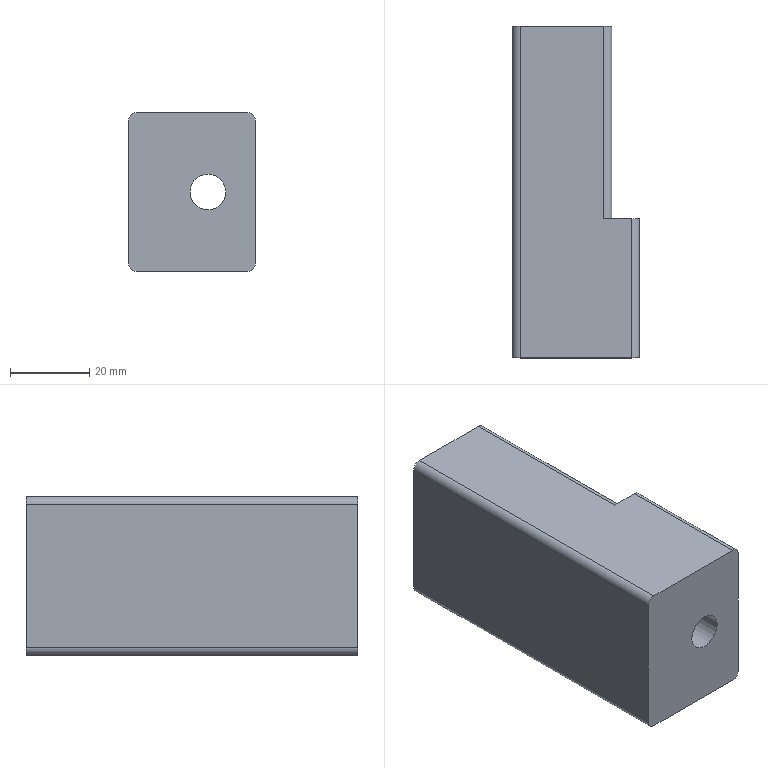NC program | Mastercam | posted with a generic post | part box 32 x 83.5 x 40 mm
Lines 1 to 1602 of 4494:
%
:0001()
(MATERIAL - ALUMINUM MM - 2024)
(T20|63 FEM |H20)
(T9|10 FEM |H9|XY STOCK TO LEAVE - .1|Z STOCK TO LEAVE - 0.)
(T10|10 FEM |H10)
(T18|10 BNOS |H18)
(T15|3 BM/BNOS |H15)
(T5|4 CHM |H5)
(T12|12 FEM |H12|XY STOCK TO LEAVE - .1|Z STOCK TO LEAVE - .1)
(T1|2 FEM |H1)
(T7|6 CHM |H7)
N100 G21
N102 G0 G17 G40 G80 G90 G94 G98
N104 G0 G28 G91 Z0.
N106 G0 G28 X0. Y0.
(63 FEM |TOOL - 20|DIA. OFF. - 20|LEN. - 20|TOOL DIA. - 63.)
N108 T20 M6
N110 G0 G54 G90 X-114.3 Y0. C0. B0. S4000 M3
N112 G43 H20 Z50.
N114 Z2.
N116 G1 Z0. F600.
N118 X114.3 F1000.
N120 G0 Z50.
N122 M5
N124 G0 G28 G91 Z0.
N126 G28
N128 M01
N130 G0 G17 G40 G80 G90 G94 G98
N132 G0 G28 G91 Z0.
(10 FEM |TOOL - 9|DIA. OFF. - 9|LEN. - 9|TOOL DIA. - 10.)
N134 T9 M6
N136 G0 G54 G90 X-42.75 Y27.1 C0. B0. S10000 M3
N138 G43 H9 Z50.
N140 Z1.
N142 G1 Z0. F600.
N144 Y26.1 F5000.
N146 G3 X-41.75 Y25.1 I1.
N148 G1 X41.75 Z-.299
N150 G2 X46.85 Y20. Z-.328 J-5.1
N152 G1 Y-20. Z-.471
N154 G2 X41.75 Y-25.1 Z-.5 I-5.1
N156 G1 X-41.75 Z-.799
N158 G2 X-46.85 Y-20. Z-.828 J5.1
N160 G1 Y20. Z-.971
N162 G2 X-41.75 Y25.1 Z-1. I5.1
N164 G1 X41.75 Z-1.299
N166 G2 X46.85 Y20. Z-1.328 J-5.1
N168 G1 Y-20. Z-1.471
N170 G2 X41.75 Y-25.1 Z-1.5 I-5.1
N172 G1 X-41.75 Z-1.799
N174 G2 X-46.85 Y-20. Z-1.828 J5.1
N176 G1 Y20. Z-1.971
N178 G2 X-41.75 Y25.1 Z-2. I5.1
N180 G1 X41.75 Z-2.299
N182 G2 X46.85 Y20. Z-2.328 J-5.1
N184 G1 Y-20. Z-2.471
N186 G2 X41.75 Y-25.1 Z-2.5 I-5.1
N188 G1 X-41.75 Z-2.799
N190 G2 X-46.85 Y-20. Z-2.828 J5.1
N192 G1 Y20. Z-2.971
N194 G2 X-41.75 Y25.1 Z-3. I5.1
N196 G1 X41.75 Z-3.299
N198 G2 X46.85 Y20. Z-3.328 J-5.1
N200 G1 Y-20. Z-3.471
N202 G2 X41.75 Y-25.1 Z-3.5 I-5.1
N204 G1 X-41.75 Z-3.799
N206 G2 X-46.85 Y-20. Z-3.828 J5.1
N208 G1 Y20. Z-3.971
N210 G2 X-41.75 Y25.1 Z-4. I5.1
N212 G1 X41.75 Z-4.299
N214 G2 X46.85 Y20. Z-4.328 J-5.1
N216 G1 Y-20. Z-4.471
N218 G2 X41.75 Y-25.1 Z-4.5 I-5.1
N220 G1 X-41.75 Z-4.799
N222 G2 X-46.85 Y-20. Z-4.828 J5.1
N224 G1 Y20. Z-4.971
N226 G2 X-41.75 Y25.1 Z-5. I5.1
N228 G1 X41.75 Z-5.299
N230 G2 X46.85 Y20. Z-5.328 J-5.1
N232 G1 Y-20. Z-5.471
N234 G2 X41.75 Y-25.1 Z-5.5 I-5.1
N236 G1 X-41.75 Z-5.799
N238 G2 X-46.85 Y-20. Z-5.828 J5.1
N240 G1 Y20. Z-5.971
N242 G2 X-41.75 Y25.1 Z-6. I5.1
N244 G1 X41.75 Z-6.299
N246 G2 X46.85 Y20. Z-6.328 J-5.1
N248 G1 Y-20. Z-6.471
N250 G2 X41.75 Y-25.1 Z-6.5 I-5.1
N252 G1 X-41.75 Z-6.799
N254 G2 X-46.85 Y-20. Z-6.828 J5.1
N256 G1 Y20. Z-6.971
N258 G2 X-41.75 Y25.1 Z-7. I5.1
N260 G1 X41.75 Z-7.299
N262 G2 X46.85 Y20. Z-7.328 J-5.1
N264 G1 Y-20. Z-7.471
N266 G2 X41.75 Y-25.1 Z-7.5 I-5.1
N268 G1 X-41.75 Z-7.799
N270 G2 X-46.85 Y-20. Z-7.828 J5.1
N272 G1 Y20. Z-7.971
N274 G2 X-41.75 Y25.1 Z-8. I5.1
N276 G1 X41.75 Z-8.299
N278 G2 X46.85 Y20. Z-8.328 J-5.1
N280 G1 Y-20. Z-8.471
N282 G2 X41.75 Y-25.1 Z-8.5 I-5.1
N284 G1 X-41.75 Z-8.799
N286 G2 X-46.85 Y-20. Z-8.828 J5.1
N288 G1 Y20. Z-8.971
N290 G2 X-41.75 Y25.1 Z-9. I5.1
N292 G1 X41.75 Z-9.299
N294 G2 X46.85 Y20. Z-9.328 J-5.1
N296 G1 Y-20. Z-9.471
N298 G2 X41.75 Y-25.1 Z-9.5 I-5.1
N300 G1 X-41.75 Z-9.799
N302 G2 X-46.85 Y-20. Z-9.828 J5.1
N304 G1 Y20. Z-9.971
N306 G2 X-41.75 Y25.1 Z-10. I5.1
N308 G1 X41.75 Z-10.299
N310 G2 X46.85 Y20. Z-10.328 J-5.1
N312 G1 Y-20. Z-10.471
N314 G2 X41.75 Y-25.1 Z-10.5 I-5.1
N316 G1 X-41.75 Z-10.799
N318 G2 X-46.85 Y-20. Z-10.828 J5.1
N320 G1 Y20. Z-10.971
N322 G2 X-41.75 Y25.1 Z-11. I5.1
N324 G1 X41.75 Z-11.299
N326 G2 X46.85 Y20. Z-11.328 J-5.1
N328 G1 Y-20. Z-11.471
N330 G2 X41.75 Y-25.1 Z-11.5 I-5.1
N332 G1 X-41.75 Z-11.799
N334 G2 X-46.85 Y-20. Z-11.828 J5.1
N336 G1 Y20. Z-11.971
N338 G2 X-41.75 Y25.1 Z-12. I5.1
N340 G1 X41.75 Z-12.299
N342 G2 X46.85 Y20. Z-12.328 J-5.1
N344 G1 Y-20. Z-12.471
N346 G2 X41.75 Y-25.1 Z-12.5 I-5.1
N348 G1 X-41.75 Z-12.799
N350 G2 X-46.85 Y-20. Z-12.828 J5.1
N352 G1 Y20. Z-12.971
N354 G2 X-41.75 Y25.1 Z-13. I5.1
N356 G1 X41.75 Z-13.299
N358 G2 X46.85 Y20. Z-13.328 J-5.1
N360 G1 Y-20. Z-13.471
N362 G2 X41.75 Y-25.1 Z-13.5 I-5.1
N364 G1 X-41.75 Z-13.799
N366 G2 X-46.85 Y-20. Z-13.828 J5.1
N368 G1 Y20. Z-13.971
N370 G2 X-41.75 Y25.1 Z-14. I5.1
N372 G1 X41.75 Z-14.299
N374 G2 X46.85 Y20. Z-14.328 J-5.1
N376 G1 Y-20. Z-14.471
N378 G2 X41.75 Y-25.1 Z-14.5 I-5.1
N380 G1 X-41.75 Z-14.799
N382 G2 X-46.85 Y-20. Z-14.828 J5.1
N384 G1 Y20. Z-14.971
N386 G2 X-41.75 Y25.1 Z-15. I5.1
N388 G1 X41.75 Z-15.299
N390 G2 X46.85 Y20. Z-15.328 J-5.1
N392 G1 Y-20. Z-15.471
N394 G2 X41.75 Y-25.1 Z-15.5 I-5.1
N396 G1 X-41.75 Z-15.799
N398 G2 X-46.85 Y-20. Z-15.828 J5.1
N400 G1 Y20. Z-15.971
N402 G2 X-41.75 Y25.1 Z-16. I5.1
N404 G1 X41.75 Z-16.299
N406 G2 X46.85 Y20. Z-16.328 J-5.1
N408 G1 Y-20. Z-16.471
N410 G2 X41.75 Y-25.1 Z-16.5 I-5.1
N412 G1 X-41.75 Z-16.799
N414 G2 X-46.85 Y-20. Z-16.828 J5.1
N416 G1 Y20. Z-16.971
N418 G2 X-41.75 Y25.1 Z-17. I5.1
N420 G1 X41.75 Z-17.299
N422 G2 X46.85 Y20. Z-17.328 J-5.1
N424 G1 Y-20. Z-17.471
N426 G2 X41.75 Y-25.1 Z-17.5 I-5.1
N428 G1 X-41.75 Z-17.799
N430 G2 X-46.85 Y-20. Z-17.828 J5.1
N432 G1 Y20. Z-17.971
N434 G2 X-41.75 Y25.1 Z-18. I5.1
N436 G1 X41.75 Z-18.299
N438 G2 X46.85 Y20. Z-18.328 J-5.1
N440 G1 Y-20. Z-18.471
N442 G2 X41.75 Y-25.1 Z-18.5 I-5.1
N444 G1 X-41.75 Z-18.799
N446 G2 X-46.85 Y-20. Z-18.828 J5.1
N448 G1 Y20. Z-18.971
N450 G2 X-41.75 Y25.1 Z-19. I5.1
N452 G1 X41.75 Z-19.299
N454 G2 X46.85 Y20. Z-19.328 J-5.1
N456 G1 Y-20. Z-19.471
N458 G2 X41.75 Y-25.1 Z-19.5 I-5.1
N460 G1 X-41.75 Z-19.799
N462 G2 X-46.85 Y-20. Z-19.828 J5.1
N464 G1 Y20. Z-19.971
N466 G2 X-41.75 Y25.1 Z-20. I5.1
N468 G1 X41.75 Z-20.299
N470 G2 X46.85 Y20. Z-20.328 J-5.1
N472 G1 Y-20. Z-20.471
N474 G2 X41.75 Y-25.1 Z-20.5 I-5.1
N476 G1 X-41.75 Z-20.799
N478 G2 X-46.85 Y-20. Z-20.828 J5.1
N480 G1 Y20. Z-20.971
N482 G2 X-41.75 Y25.1 Z-21. I5.1
N484 G1 X41.75 Z-21.299
N486 G2 X46.85 Y20. Z-21.328 J-5.1
N488 G1 Y-20. Z-21.471
N490 G2 X41.75 Y-25.1 Z-21.5 I-5.1
N492 G1 X-41.75 Z-21.799
N494 G2 X-46.85 Y-20. Z-21.828 J5.1
N496 G1 Y20. Z-21.971
N498 G2 X-41.75 Y25.1 Z-22. I5.1
N500 G1 X41.75 Z-22.299
N502 G2 X46.85 Y20. Z-22.328 J-5.1
N504 G1 Y-20. Z-22.471
N506 G2 X41.75 Y-25.1 Z-22.5 I-5.1
N508 G1 X-41.75 Z-22.799
N510 G2 X-46.85 Y-20. Z-22.828 J5.1
N512 G1 Y20. Z-22.971
N514 G2 X-41.75 Y25.1 Z-23. I5.1
N516 G1 X41.75 Z-23.299
N518 G2 X46.85 Y20. Z-23.328 J-5.1
N520 G1 Y-20. Z-23.471
N522 G2 X41.75 Y-25.1 Z-23.5 I-5.1
N524 G1 X-41.75 Z-23.799
N526 G2 X-46.85 Y-20. Z-23.828 J5.1
N528 G1 Y20. Z-23.971
N530 G2 X-41.75 Y25.1 Z-24. I5.1
N532 G1 X41.75 Z-24.299
N534 G2 X46.85 Y20. Z-24.328 J-5.1
N536 G1 Y-20. Z-24.471
N538 G2 X41.75 Y-25.1 Z-24.5 I-5.1
N540 G1 X-41.75 Z-24.799
N542 G2 X-46.85 Y-20. Z-24.828 J5.1
N544 G1 Y20. Z-24.971
N546 G2 X-41.75 Y25.1 Z-25. I5.1
N548 G1 X41.75 Z-25.299
N550 G2 X46.85 Y20. Z-25.328 J-5.1
N552 G1 Y-20. Z-25.471
N554 G2 X41.75 Y-25.1 Z-25.5 I-5.1
N556 G1 X-41.75 Z-25.799
N558 G2 X-46.85 Y-20. Z-25.828 J5.1
N560 G1 Y20. Z-25.971
N562 G2 X-41.75 Y25.1 Z-26. I5.1
N564 G1 X41.75 Z-26.299
N566 G2 X46.85 Y20. Z-26.328 J-5.1
N568 G1 Y-20. Z-26.471
N570 G2 X41.75 Y-25.1 Z-26.5 I-5.1
N572 G1 X-41.75 Z-26.799
N574 G2 X-46.85 Y-20. Z-26.828 J5.1
N576 G1 Y20. Z-26.971
N578 G2 X-41.75 Y25.1 Z-27. I5.1
N580 G1 X41.75 Z-27.299
N582 G2 X46.85 Y20. Z-27.328 J-5.1
N584 G1 Y-20. Z-27.471
N586 G2 X41.75 Y-25.1 Z-27.5 I-5.1
N588 G1 X-41.75 Z-27.799
N590 G2 X-46.85 Y-20. Z-27.828 J5.1
N592 G1 Y20. Z-27.971
N594 G2 X-41.75 Y25.1 Z-28. I5.1
N596 G1 X41.75 Z-28.299
N598 G2 X46.85 Y20. Z-28.328 J-5.1
N600 G1 Y-20. Z-28.471
N602 G2 X41.75 Y-25.1 Z-28.5 I-5.1
N604 G1 X-41.75 Z-28.799
N606 G2 X-46.85 Y-20. Z-28.828 J5.1
N608 G1 Y20. Z-28.971
N610 G2 X-41.75 Y25.1 Z-29. I5.1
N612 G1 X41.75 Z-29.299
N614 G2 X46.85 Y20. Z-29.328 J-5.1
N616 G1 Y-20. Z-29.471
N618 G2 X41.75 Y-25.1 Z-29.5 I-5.1
N620 G1 X-41.75 Z-29.799
N622 G2 X-46.85 Y-20. Z-29.828 J5.1
N624 G1 Y20. Z-29.971
N626 G2 X-41.75 Y25.1 Z-30. I5.1
N628 G1 X41.75 Z-30.299
N630 G2 X46.85 Y20. Z-30.328 J-5.1
N632 G1 Y-20. Z-30.471
N634 G2 X41.75 Y-25.1 Z-30.5 I-5.1
N636 G1 X-41.75 Z-30.799
N638 G2 X-46.85 Y-20. Z-30.828 J5.1
N640 G1 Y20. Z-30.971
N642 G2 X-41.75 Y25.1 Z-31. I5.1
N644 G1 X41.75 Z-31.299
N646 G2 X46.85 Y20. Z-31.328 J-5.1
N648 G1 Y-20. Z-31.471
N650 G2 X41.75 Y-25.1 Z-31.5 I-5.1
N652 G1 X-41.75 Z-31.799
N654 G2 X-46.85 Y-20. Z-31.828 J5.1
N656 G1 Y20. Z-31.971
N658 G2 X-41.75 Y25.1 Z-32. I5.1
N660 G1 X41.75 Z-32.299
N662 G2 X46.85 Y20. Z-32.328 J-5.1
N664 G1 Y-20. Z-32.471
N666 G2 X41.75 Y-25.1 Z-32.5 I-5.1
N668 G1 X-41.75
N670 G2 X-46.85 Y-20. J5.1
N672 G1 Y20.
N674 G2 X-41.75 Y25.1 I5.1
N676 G1 X41.75
N678 G2 X46.85 Y20. J-5.1
N680 G1 Y-20.
N682 G2 X41.75 Y-25.1 I-5.1
N684 G3 X40.75 Y-26.1 J-1.
N686 G1 Y-27.1
N688 G0 Z50.
N690 M5
N692 G0 G28 G91 Z0.
N694 G28
N696 M01
N698 G0 G17 G40 G80 G90 G94 G98
N700 G0 G28 G91 Z0.
(10 FEM |TOOL - 10|DIA. OFF. - 10|LEN. - 10|TOOL DIA. - 10.)
N702 T10 M6
N704 G0 G54 G90 X-46.75 Y-25.002 C0. B0. S7000 M3
N706 G43 H10 Z50.
N708 Z1.
N710 G1 Z-16.25 F600.
N712 Y-.002 F1000.
N714 Y20.
N716 G2 X-41.75 Y25. I5.
N718 G1 X41.75
N720 G2 X46.75 Y20. J-5.
N722 G1 Y-20.
N724 G2 X41.75 Y-25. I-5.
N726 G1 X-41.75
N728 G2 X-46.75 Y-20. J5.
N730 G1 Y-.002
N732 Y24.998
N734 G0 Z50.
N736 Y-25.002
N738 Z-15.25
N740 G1 Z-32.5 F600.
N742 Y-.002 F1000.
N744 Y20.
N746 G2 X-41.75 Y25. I5.
N748 G1 X41.75
N750 G2 X46.75 Y20. J-5.
N752 G1 Y-20.
N754 G2 X41.75 Y-25. I-5.
N756 G1 X-41.75
N758 G2 X-46.75 Y-20. J5.
N760 G1 Y-.002
N762 Y24.998
N764 G0 Z50.
N766 M5
N768 G0 G28 G91 Z0.
N770 G28
N772 M01
N774 G0 G17 G40 G80 G90 G94 G98
N776 G0 G28 G91 Z0.
(10 BNOS |TOOL - 18|DIA. OFF. - 18|LEN. - 18|TOOL DIA. - 10.)
N778 T18 M6
N780 G0 G54 G90 X46.75 Y22. C0. B0. S7000 M3
N782 G43 H18 Z50.
N784 Z5.
N786 G1 Z0. F600.
N788 X41.75 F3000.
N790 X-41.75
N792 X-46.75
N794 Y22.134
N796 Z-.003
N798 X-41.75
N800 X41.75
N802 X46.75
N804 Y22.27
N806 Z-.012
N808 X41.75
N810 X-41.75
N812 X-46.75
N814 Y22.407
N816 Z-.028
N818 X-41.75
N820 X41.75
N822 X46.75
N824 Y22.546
N826 Z-.05
N828 X41.75
N830 X-41.75
N832 X-46.75
N834 Y22.686
N836 Z-.079
N838 X-41.75
N840 X41.75
N842 X46.75
N844 Y22.825
N846 Z-.116
N848 X41.75
N850 X-41.75
N852 X-46.75
N854 Y22.965
N856 Z-.16
N858 X-41.75
N860 X41.75
N862 X46.75
N864 Y23.104
N866 Z-.211
N868 X41.75
N870 X-41.75
N872 X-46.75
N874 Y23.227
N876 Z-.262
N878 X-41.75
N880 X41.75
N882 X46.75
N884 Y23.348
N886 Z-.32
N888 X41.75
N890 X-41.75
N892 X-46.75
N894 Y23.467
N896 Z-.383
N898 X-41.75
N900 X41.75
N902 X46.75
N904 Y23.584
N906 Z-.452
N908 X41.75
N910 X-41.75
N912 X-46.75
N914 Y23.698
N916 Z-.527
N918 X-41.75
N920 X41.75
N922 X46.75
N924 Y23.81
N926 Z-.607
N928 X41.75
N930 X-41.75
N932 X-46.75
N934 Y23.918
N936 Z-.693
N938 X-41.75
N940 X41.75
N942 X46.75
N944 Y24.021
N946 Z-.783
N948 X41.75
N950 X-41.75
N952 X-46.75
N954 Y24.121
N956 Z-.879
N958 X-41.75
N960 X41.75
N962 X46.75
N964 Y24.217
N966 Z-.979
N968 X41.75
N970 X-41.75
N972 X-46.75
N974 Y24.307
N976 Z-1.082
N978 X-41.75
N980 X41.75
N982 X46.75
N984 Y24.393
N986 Z-1.19
N988 X41.75
N990 X-41.75
N992 X-46.75
N994 Y24.473
N996 Z-1.302
N998 X-41.75
N1000 X41.75
N1002 X46.75
N1004 Y24.548
N1006 Z-1.416
N1008 X41.75
N1010 X-41.75
N1012 X-46.75
N1014 Y24.617
N1016 Z-1.533
N1018 X-41.75
N1020 X41.75
N1022 X46.75
N1024 Y24.68
N1026 Z-1.652
N1028 X41.75
N1030 X-41.75
N1032 X-46.75
N1034 Y24.738
N1036 Z-1.773
N1038 X-41.75
N1040 X41.75
N1042 X46.75
N1044 Y24.789
N1046 Z-1.896
N1048 X41.75
N1050 X-41.75
N1052 X-46.75
N1054 Y24.84
N1056 Z-2.035
N1058 X-41.75
N1060 X41.75
N1062 X46.75
N1064 Y24.884
N1066 Z-2.175
N1068 X41.75
N1070 X-41.75
N1072 X-46.75
N1074 Y24.921
N1076 Z-2.314
N1078 X-41.75
N1080 X41.75
N1082 X46.75
N1084 Y24.95
N1086 Z-2.454
N1088 X41.75
N1090 X-41.75
N1092 X-46.75
N1094 Y24.972
N1096 Z-2.593
N1098 X-41.75
N1100 X41.75
N1102 X46.75
N1104 Y24.988
N1106 Z-2.73
N1108 X41.75
N1110 X-41.75
N1112 X-46.75
N1114 Y24.997
N1116 Z-2.866
N1118 X-41.75
N1120 X41.75
N1122 X46.75
N1124 Y25.
N1126 Z-3.
N1128 X41.75
N1130 X-41.75
N1132 X-46.75
N1134 G0 Z2.
N1136 Z50.
N1138 Y-25.
N1140 Z2.
N1142 G1 Z-3. F600.
N1144 X-41.75 F3000.
N1146 X41.75
N1148 X46.75
N1150 Z-2.866
N1152 Y-24.997
N1154 X41.75
N1156 X-41.75
N1158 X-46.75
N1160 Z-2.73
N1162 Y-24.988
N1164 X-41.75
N1166 X41.75
N1168 X46.75
N1170 Z-2.593
N1172 Y-24.972
N1174 X41.75
N1176 X-41.75
N1178 X-46.75
N1180 Z-2.454
N1182 Y-24.95
N1184 X-41.75
N1186 X41.75
N1188 X46.75
N1190 Z-2.314
N1192 Y-24.921
N1194 X41.75
N1196 X-41.75
N1198 X-46.75
N1200 Z-2.175
N1202 Y-24.884
N1204 X-41.75
N1206 X41.75
N1208 X46.75
N1210 Z-2.035
N1212 Y-24.84
N1214 X41.75
N1216 X-41.75
N1218 X-46.75
N1220 Z-1.896
N1222 Y-24.789
N1224 X-41.75
N1226 X41.75
N1228 X46.75
N1230 Z-1.773
N1232 Y-24.738
N1234 X41.75
N1236 X-41.75
N1238 X-46.75
N1240 Z-1.652
N1242 Y-24.68
N1244 X-41.75
N1246 X41.75
N1248 X46.75
N1250 Z-1.533
N1252 Y-24.617
N1254 X41.75
N1256 X-41.75
N1258 X-46.75
N1260 Z-1.416
N1262 Y-24.548
N1264 X-41.75
N1266 X41.75
N1268 X46.75
N1270 Z-1.302
N1272 Y-24.473
N1274 X41.75
N1276 X-41.75
N1278 X-46.75
N1280 Z-1.19
N1282 Y-24.393
N1284 X-41.75
N1286 X41.75
N1288 X46.75
N1290 Z-1.082
N1292 Y-24.307
N1294 X41.75
N1296 X-41.75
N1298 X-46.75
N1300 Z-.979
N1302 Y-24.217
N1304 X-41.75
N1306 X41.75
N1308 X46.75
N1310 Z-.879
N1312 Y-24.121
N1314 X41.75
N1316 X-41.75
N1318 X-46.75
N1320 Z-.783
N1322 Y-24.021
N1324 X-41.75
N1326 X41.75
N1328 X46.75
N1330 Z-.693
N1332 Y-23.918
N1334 X41.75
N1336 X-41.75
N1338 X-46.75
N1340 Z-.607
N1342 Y-23.81
N1344 X-41.75
N1346 X41.75
N1348 X46.75
N1350 Z-.527
N1352 Y-23.698
N1354 X41.75
N1356 X-41.75
N1358 X-46.75
N1360 Z-.452
N1362 Y-23.584
N1364 X-41.75
N1366 X41.75
N1368 X46.75
N1370 Z-.383
N1372 Y-23.467
N1374 X41.75
N1376 X-41.75
N1378 X-46.75
N1380 Z-.32
N1382 Y-23.348
N1384 X-41.75
N1386 X41.75
N1388 X46.75
N1390 Z-.262
N1392 Y-23.227
N1394 X41.75
N1396 X-41.75
N1398 X-46.75
N1400 Z-.211
N1402 Y-23.104
N1404 X-41.75
N1406 X41.75
N1408 X46.75
N1410 Z-.16
N1412 Y-22.965
N1414 X41.75
N1416 X-41.75
N1418 X-46.75
N1420 Z-.116
N1422 Y-22.825
N1424 X-41.75
N1426 X41.75
N1428 X46.75
N1430 Z-.079
N1432 Y-22.686
N1434 X41.75
N1436 X-41.75
N1438 X-46.75
N1440 Z-.05
N1442 Y-22.546
N1444 X-41.75
N1446 X41.75
N1448 X46.75
N1450 Z-.028
N1452 Y-22.407
N1454 X41.75
N1456 X-41.75
N1458 X-46.75
N1460 Z-.012
N1462 Y-22.27
N1464 X-41.75
N1466 X41.75
N1468 X46.75
N1470 Z-.003
N1472 Y-22.134
N1474 X41.75
N1476 X-41.75
N1478 X-46.75
N1480 Z0.
N1482 Y-22.
N1484 X-41.75
N1486 X41.75
N1488 X46.75
N1490 G0 Z5.
N1492 Z50.
N1494 M5
N1496 G0 G28 G91 Z0.
N1498 G28
N1500 M01
N1502 G0 G17 G40 G80 G90 G94 G98
N1504 G0 G28 G91 Z0.
(3 BM/BNOS |TOOL - 15|DIA. OFF. - 15|LEN. - 15|TOOL DIA. - 3.)
N1506 T15 M6
N1508 G0 G54 G90 X43.906 Y22.212 C0. B0. S7000 M3
N1510 G43 H15 Z50.
N1512 Z16.225
N1514 Z6.225
N1516 G1 Z-3.775 F600.
N1518 X43.887 Y22.194 Z-3.92 F1000.
N1520 X43.836 Y22.142 Z-4.051
N1522 X43.758 Y22.064 Z-4.167
N1524 X43.66 Y21.966 Z-4.266
N1526 X43.548 Y21.855 Z-4.347
N1528 X43.43 Y21.737 Z-4.407
N1530 X43.311 Y21.618 Z-4.445
N1532 X43.199 Y21.506 Z-4.46
N1534 X43.096 Y21.401 Z-4.437
N1536 X43.003 Y21.304 Z-4.366
N1538 X42.922 Y21.217 Z-4.259
N1540 X42.853 Y21.14 Z-4.122
N1542 X42.797 Y21.075 Z-3.967
N1544 X42.756 Y21.024 Z-3.801
N1546 X42.73 Y20.988 Z-3.634
N1548 X42.72 Y20.969 Z-3.475
N1550 X42.719 Y20.959 Z-3.327
N1552 X42.72 Y20.956 Z-3.253
N1554 X42.719 Y20.951 Z-3.179
N1556 Y20.927 Z-3.029
N1558 X42.72 Y20.915 Z-2.954
N1560 X42.719 Y20.902 Z-2.88
N1562 X42.721 Y20.864 Z-2.731
N1564 X42.72 Y20.823 Z-2.582
N1566 X42.721 Y20.768 Z-2.438
N1568 Y20.712 Z-2.294
N1570 Y20.642 Z-2.156
N1572 Y20.572 Z-2.018
N1574 Y20.488 Z-1.888
N1576 Y20.402 Z-1.757
N1578 Y20.305 Z-1.636
N1580 X42.72 Y20.206 Z-1.515
N1582 X42.721 Y20.096 Z-1.404
N1584 X42.72 Y19.985 Z-1.294
N1586 X42.721 Y19.864 Z-1.195
N1588 Y19.743 Z-1.098
N1590 Y19.613 Z-1.012
N1592 Y19.482 Z-.928
N1594 Y19.344 Z-.858
N1596 Y19.206 Z-.788
N1598 Y19.062 Z-.732
N1600 X42.72 Y18.918 Z-.677
N1602 X42.721 Y18.769 Z-.636
N1604 X42.719 Y18.62 Z-.598
N1606 X42.72 Y18.546 Z-.585
N1608 X42.719 Y18.471 Z-.573
N1610 Y18.321 Z-.549
N1612 X42.72 Y18.247 Z-.544
N1614 X42.719 Y18.173 Z-.541
N1616 Y18.025 Z-.531
N1618 Y16.8
N1620 Y15.6
N1622 Y14.4
N1624 Y13.2
N1626 Y12.
N1628 Y10.8
N1630 Y9.6
N1632 Y8.4
N1634 Y7.2
N1636 Y6.
N1638 Y4.8
N1640 Y3.6
N1642 Y2.4
N1644 Y1.2
N1646 Y0.
N1648 Y-1.2
N1650 Y-2.4
N1652 Y-3.6
N1654 Y-4.8
N1656 Y-6.
N1658 Y-7.2
N1660 Y-8.4
N1662 Y-9.6
N1664 Y-10.8
N1666 Y-12.
N1668 Y-13.2
N1670 Y-14.4
N1672 Y-15.6
N1674 Y-16.8
N1676 X42.72 Y-18.025
N1678 X42.719 Y-18.173 Z-.541
N1680 X42.72 Y-18.247 Z-.544
N1682 X42.719 Y-18.321 Z-.549
N1684 Y-18.471 Z-.573
N1686 X42.72 Y-18.546 Z-.585
N1688 X42.719 Y-18.62 Z-.598
N1690 X42.721 Y-18.769 Z-.636
N1692 X42.72 Y-18.918 Z-.677
N1694 X42.721 Y-19.062 Z-.732
N1696 Y-19.206 Z-.788
N1698 Y-19.344 Z-.858
N1700 Y-19.482 Z-.928
N1702 Y-19.612 Z-1.012
N1704 Y-19.743 Z-1.098
N1706 Y-19.864 Z-1.195
N1708 X42.72 Y-19.985 Z-1.294
N1710 X42.721 Y-20.096 Z-1.404
N1712 X42.72 Y-20.206 Z-1.515
N1714 X42.721 Y-20.305 Z-1.636
N1716 Y-20.402 Z-1.757
N1718 Y-20.488 Z-1.888
N1720 Y-20.572 Z-2.018
N1722 Y-20.642 Z-2.156
N1724 Y-20.712 Z-2.294
N1726 Y-20.768 Z-2.438
N1728 X42.72 Y-20.823 Z-2.582
N1730 X42.721 Y-20.864 Z-2.731
N1732 X42.719 Y-20.902 Z-2.88
N1734 X42.72 Y-20.915 Z-2.954
N1736 X42.719 Y-20.927 Z-3.029
N1738 Y-20.951 Z-3.179
N1740 X42.72 Y-20.956 Z-3.253
N1742 X42.719 Y-20.959 Z-3.327
N1744 Y-20.968 Z-3.475
N1746 X42.728 Y-20.986 Z-3.633
N1748 X42.753 Y-21.021 Z-3.8
N1750 X42.793 Y-21.071 Z-3.966
N1752 X42.848 Y-21.135 Z-4.122
N1754 X42.917 Y-21.212 Z-4.259
N1756 X42.997 Y-21.299 Z-4.367
N1758 X43.089 Y-21.395 Z-4.437
N1760 X43.192 Y-21.499 Z-4.461
N1762 X43.304 Y-21.611 Z-4.446
N1764 X43.423 Y-21.73 Z-4.407
N1766 X43.541 Y-21.848 Z-4.347
N1768 X43.653 Y-21.959 Z-4.267
N1770 X43.751 Y-22.057 Z-4.168
N1772 X43.829 Y-22.135 Z-4.052
N1774 X43.881 Y-22.187 Z-3.92
N1776 X43.899 Y-22.206 Z-3.775
N1778 G0 Z6.225
N1780 Z16.225
N1782 Z50.
N1784 X-43.896 Y-22.202
N1786 Z16.224
N1788 Z6.224
N1790 G1 Z-3.776 F600.
N1792 X-43.877 Y-22.183 Z-3.921 F1000.
N1794 X-43.825 Y-22.132 Z-4.052
N1796 X-43.747 Y-22.054 Z-4.168
N1798 X-43.649 Y-21.956 Z-4.267
N1800 X-43.538 Y-21.844 Z-4.347
N1802 X-43.419 Y-21.726 Z-4.407
N1804 X-43.301 Y-21.608 Z-4.446
N1806 X-43.188 Y-21.495 Z-4.461
N1808 X-43.086 Y-21.392 Z-4.437
N1810 X-42.994 Y-21.296 Z-4.367
N1812 X-42.914 Y-21.209 Z-4.258
N1814 X-42.846 Y-21.133 Z-4.122
N1816 X-42.792 Y-21.07 Z-3.966
N1818 X-42.752 Y-21.02 Z-3.8
N1820 X-42.728 Y-20.986 Z-3.633
N1822 X-42.719 Y-20.969 Z-3.475
N1824 X-42.72 Y-20.961 Z-3.327
N1826 Y-20.956 Z-3.253
N1828 X-42.719 Y-20.951 Z-3.179
N1830 X-42.72 Y-20.928 Z-3.029
N1832 Y-20.916 Z-2.954
N1834 Y-20.903 Z-2.879
N1836 X-42.721 Y-20.864 Z-2.731
N1838 X-42.72 Y-20.823 Z-2.582
N1840 X-42.721 Y-20.768 Z-2.438
N1842 Y-20.712 Z-2.294
N1844 Y-20.642 Z-2.156
N1846 Y-20.572 Z-2.018
N1848 Y-20.488 Z-1.888
N1850 Y-20.402 Z-1.757
N1852 Y-20.305 Z-1.636
N1854 X-42.72 Y-20.206 Z-1.515
N1856 X-42.721 Y-20.096 Z-1.404
N1858 X-42.72 Y-19.985 Z-1.294
N1860 X-42.721 Y-19.864 Z-1.195
N1862 Y-19.743 Z-1.098
N1864 Y-19.612 Z-1.012
N1866 Y-19.482 Z-.928
N1868 Y-19.344 Z-.858
N1870 Y-19.206 Z-.788
N1872 Y-19.062 Z-.732
N1874 X-42.72 Y-18.918 Z-.677
N1876 X-42.721 Y-18.769 Z-.636
N1878 X-42.72 Y-18.621 Z-.597
N1880 Y-18.546 Z-.584
N1882 Y-18.471 Z-.572
N1884 X-42.719 Y-18.321 Z-.549
N1886 X-42.72 Y-18.247 Z-.544
N1888 Y-18.173 Z-.539
N1890 X-42.719 Y-18.025 Z-.531
N1892 Y-16.759
N1894 Y-15.517
N1896 Y-14.276
N1898 Y-13.034
N1900 Y-11.793
N1902 Y-10.552
N1904 Y-9.31
N1906 Y-8.069
N1908 Y-6.828
N1910 Y-5.586
N1912 Y-4.345
N1914 Y-3.103
N1916 Y-1.862
N1918 Y-.621
N1920 Y.621
N1922 Y1.862
N1924 Y3.103
N1926 Y4.345
N1928 Y5.586
N1930 Y6.828
N1932 Y8.069
N1934 Y9.31
N1936 Y10.552
N1938 Y11.793
N1940 Y13.034
N1942 Y14.276
N1944 Y15.517
N1946 Y16.759
N1948 Y18.025
N1950 X-42.72 Y18.173 Z-.539
N1952 Y18.247 Z-.544
N1954 X-42.719 Y18.321 Z-.549
N1956 X-42.72 Y18.471 Z-.572
N1958 Y18.546 Z-.584
N1960 Y18.621 Z-.597
N1962 X-42.721 Y18.769 Z-.636
N1964 X-42.72 Y18.918 Z-.677
N1966 X-42.721 Y19.062 Z-.732
N1968 Y19.206 Z-.788
N1970 Y19.344 Z-.858
N1972 Y19.482 Z-.928
N1974 Y19.612 Z-1.012
N1976 Y19.743 Z-1.098
N1978 Y19.864 Z-1.195
N1980 X-42.72 Y19.985 Z-1.294
N1982 X-42.721 Y20.096 Z-1.404
N1984 X-42.72 Y20.206 Z-1.515
N1986 X-42.721 Y20.305 Z-1.636
N1988 Y20.402 Z-1.757
N1990 Y20.488 Z-1.888
N1992 Y20.572 Z-2.018
N1994 Y20.642 Z-2.156
N1996 Y20.712 Z-2.294
N1998 Y20.768 Z-2.438
N2000 X-42.72 Y20.823 Z-2.582
N2002 X-42.721 Y20.864 Z-2.731
N2004 X-42.72 Y20.903 Z-2.879
N2006 Y20.916 Z-2.954
N2008 Y20.928 Z-3.029
N2010 X-42.719 Y20.951 Z-3.179
N2012 X-42.72 Y20.956 Z-3.253
N2014 Y20.961 Z-3.327
N2016 X-42.719 Y20.969 Z-3.475
N2018 X-42.728 Y20.986 Z-3.633
N2020 X-42.752 Y21.02 Z-3.8
N2022 X-42.792 Y21.07 Z-3.966
N2024 X-42.846 Y21.133 Z-4.122
N2026 X-42.914 Y21.209 Z-4.258
N2028 X-42.994 Y21.296 Z-4.367
N2030 X-43.086 Y21.392 Z-4.437
N2032 X-43.188 Y21.495 Z-4.461
N2034 X-43.301 Y21.608 Z-4.446
N2036 X-43.419 Y21.726 Z-4.407
N2038 X-43.538 Y21.844 Z-4.347
N2040 X-43.649 Y21.956 Z-4.267
N2042 X-43.747 Y22.054 Z-4.168
N2044 X-43.825 Y22.132 Z-4.052
N2046 X-43.877 Y22.183 Z-3.921
N2048 X-43.896 Y22.202 Z-3.776
N2050 G0 Z6.224
N2052 Z16.224
N2054 Z50.
N2056 M5
N2058 G0 G28 G91 Z0.
N2060 G28
N2062 M01
N2064 G0 G17 G40 G80 G90 G94 G98
N2066 G0 G28 G91 Z0.
(63 FEM |TOOL - 20|DIA. OFF. - 20|LEN. - 20|TOOL DIA. - 63.)
N2068 T20 M6
N2070 G0 G54 G90 X-114.3 Y0. C0. B0. S4000 M3
N2072 G43 H20 Z55.
N2074 Z7.
N2076 G1 Z4.51 F600.
N2078 X114.3 F3000.
N2080 G0 Z54.51
N2082 X-114.3
N2084 Z6.51
N2086 G1 Z4.02 F600.
N2088 X114.3 F3000.
N2090 G0 Z54.02
N2092 X-114.3
N2094 Z6.02
N2096 G1 Z3.53 F600.
N2098 X114.3 F3000.
N2100 G0 Z53.53
N2102 X-114.3
N2104 Z5.53
N2106 G1 Z3.04 F600.
N2108 X114.3 F3000.
N2110 G0 Z53.04
N2112 X-114.3
N2114 Z5.04
N2116 G1 Z2.55 F600.
N2118 X114.3 F3000.
N2120 G0 Z52.55
N2122 X-114.3
N2124 Z4.55
N2126 G1 Z2.06 F600.
N2128 X114.3 F3000.
N2130 G0 Z52.06
N2132 X-114.3
N2134 Z4.06
N2136 G1 Z1.57 F600.
N2138 X114.3 F3000.
N2140 G0 Z51.57
N2142 X-114.3
N2144 Z3.57
N2146 G1 Z1.08 F600.
N2148 X114.3 F3000.
N2150 G0 Z51.08
N2152 X-114.3
N2154 Z3.08
N2156 G1 Z.59 F600.
N2158 X114.3 F3000.
N2160 G0 Z50.59
N2162 X-114.3
N2164 Z2.59
N2166 G1 Z.1 F600.
N2168 X114.3 F3000.
N2170 G0 Z50.1
N2172 X-114.3
N2174 Z2.1
N2176 G1 Z0. F600.
N2178 X114.3 F1000.
N2180 G0 Z50.
N2182 M5
N2184 G0 G28 G91 Z0.
N2186 G28
N2188 M01
N2190 G0 G17 G40 G80 G90 G94 G98
N2192 G0 G28 G91 Z0.
(10 BNOS |TOOL - 18|DIA. OFF. - 18|LEN. - 18|TOOL DIA. - 10.)
N2194 T18 M6
N2196 G0 G54 G90 X-1.75 Y22. C0. B0. S7000 M3
N2198 G43 H18 Z50.
N2200 Z5.
N2202 G1 Z0. F600.
N2204 X-6.75 F3000.
N2206 X-41.75
N2208 X-46.75
N2210 Y22.134
N2212 Z-.003
N2214 X-41.75
N2216 X-6.75
N2218 X-1.75
N2220 Y22.27
N2222 Z-.012
N2224 X-6.75
N2226 X-41.75
N2228 X-46.75
N2230 Y22.407
N2232 Z-.028
N2234 X-41.75
N2236 X-6.75
N2238 X-1.75
N2240 Y22.546
N2242 Z-.05
N2244 X-6.75
N2246 X-41.75
N2248 X-46.75
N2250 Y22.686
N2252 Z-.079
N2254 X-41.75
N2256 X-6.75
N2258 X-1.75
N2260 Y22.825
N2262 Z-.116
N2264 X-6.75
N2266 X-41.75
N2268 X-46.75
N2270 Y22.965
N2272 Z-.16
N2274 X-41.75
N2276 X-6.75
N2278 X-1.75
N2280 Y23.104
N2282 Z-.211
N2284 X-6.75
N2286 X-41.75
N2288 X-46.75
N2290 Y23.227
N2292 Z-.262
N2294 X-41.75
N2296 X-6.75
N2298 X-1.75
N2300 Y23.348
N2302 Z-.32
N2304 X-6.75
N2306 X-41.75
N2308 X-46.75
N2310 Y23.467
N2312 Z-.383
N2314 X-41.75
N2316 X-6.75
N2318 X-1.75
N2320 Y23.584
N2322 Z-.452
N2324 X-6.75
N2326 X-41.75
N2328 X-46.75
N2330 Y23.698
N2332 Z-.527
N2334 X-41.75
N2336 X-6.75
N2338 X-1.75
N2340 Y23.81
N2342 Z-.607
N2344 X-6.75
N2346 X-41.75
N2348 X-46.75
N2350 Y23.918
N2352 Z-.693
N2354 X-41.75
N2356 X-6.75
N2358 X-1.75
N2360 Y24.021
N2362 Z-.783
N2364 X-6.75
N2366 X-41.75
N2368 X-46.75
N2370 Y24.121
N2372 Z-.879
N2374 X-41.75
N2376 X-6.75
N2378 X-1.75
N2380 Y24.217
N2382 Z-.979
N2384 X-6.75
N2386 X-41.75
N2388 X-46.75
N2390 Y24.307
N2392 Z-1.082
N2394 X-41.75
N2396 X-6.75
N2398 X-1.75
N2400 Y24.393
N2402 Z-1.19
N2404 X-6.75
N2406 X-41.75
N2408 X-46.75
N2410 Y24.473
N2412 Z-1.302
N2414 X-41.75
N2416 X-6.75
N2418 X-1.75
N2420 Y24.548
N2422 Z-1.416
N2424 X-6.75
N2426 X-41.75
N2428 X-46.75
N2430 Y24.617
N2432 Z-1.533
N2434 X-41.75
N2436 X-6.75
N2438 X-1.75
N2440 Y24.68
N2442 Z-1.652
N2444 X-6.75
N2446 X-41.75
N2448 X-46.75
N2450 Y24.738
N2452 Z-1.773
N2454 X-41.75
N2456 X-6.75
N2458 X-1.75
N2460 Y24.789
N2462 Z-1.896
N2464 X-6.75
N2466 X-41.75
N2468 X-46.75
N2470 Y24.84
N2472 Z-2.035
N2474 X-41.75
N2476 X-6.75
N2478 X-1.75
N2480 Y24.884
N2482 Z-2.175
N2484 X-6.75
N2486 X-41.75
N2488 X-46.75
N2490 Y24.921
N2492 Z-2.314
N2494 X-41.75
N2496 X-6.75
N2498 X-1.75
N2500 Y24.95
N2502 Z-2.454
N2504 X-6.75
N2506 X-41.75
N2508 X-46.75
N2510 Y24.972
N2512 Z-2.593
N2514 X-41.75
N2516 X-6.75
N2518 X-1.75
N2520 Y24.988
N2522 Z-2.73
N2524 X-6.75
N2526 X-41.75
N2528 X-46.75
N2530 Y24.997
N2532 Z-2.866
N2534 X-41.75
N2536 X-6.75
N2538 X-1.75
N2540 Y25.
N2542 Z-3.
N2544 X-6.75
N2546 X-41.75
N2548 X-46.75
N2550 G0 Z2.
N2552 Z50.
N2554 Y-25.
N2556 Z2.
N2558 G1 Z-3. F600.
N2560 X-41.75 F3000.
N2562 X-6.75
N2564 X-1.75
N2566 Z-2.866
N2568 Y-24.997
N2570 X-6.75
N2572 X-41.75
N2574 X-46.75
N2576 Z-2.73
N2578 Y-24.988
N2580 X-41.75
N2582 X-6.75
N2584 X-1.75
N2586 Z-2.593
N2588 Y-24.972
N2590 X-6.75
N2592 X-41.75
N2594 X-46.75
N2596 Z-2.454
N2598 Y-24.95
N2600 X-41.75
N2602 X-6.75
N2604 X-1.75
N2606 Z-2.314
N2608 Y-24.921
N2610 X-6.75
N2612 X-41.75
N2614 X-46.75
N2616 Z-2.175
N2618 Y-24.884
N2620 X-41.75
N2622 X-6.75
N2624 X-1.75
N2626 Z-2.035
N2628 Y-24.84
N2630 X-6.75
N2632 X-41.75
N2634 X-46.75
N2636 Z-1.896
N2638 Y-24.789
N2640 X-41.75
N2642 X-6.75
N2644 X-1.75
N2646 Z-1.773
N2648 Y-24.738
N2650 X-6.75
N2652 X-41.75
N2654 X-46.75
N2656 Z-1.652
N2658 Y-24.68
N2660 X-41.75
N2662 X-6.75
N2664 X-1.75
N2666 Z-1.533
N2668 Y-24.617
N2670 X-6.75
N2672 X-41.75
N2674 X-46.75
N2676 Z-1.416
N2678 Y-24.548
N2680 X-41.75
N2682 X-6.75
N2684 X-1.75
N2686 Z-1.302
N2688 Y-24.473
N2690 X-6.75
N2692 X-41.75
N2694 X-46.75
N2696 Z-1.19
N2698 Y-24.393
N2700 X-41.75
N2702 X-6.75
N2704 X-1.75
N2706 Z-1.082
N2708 Y-24.307
N2710 X-6.75
N2712 X-41.75
N2714 X-46.75
N2716 Z-.979
N2718 Y-24.217
N2720 X-41.75
N2722 X-6.75
N2724 X-1.75
N2726 Z-.879
N2728 Y-24.121
N2730 X-6.75
N2732 X-41.75
N2734 X-46.75
N2736 Z-.783
N2738 Y-24.021
N2740 X-41.75
N2742 X-6.75
N2744 X-1.75
N2746 Z-.693
N2748 Y-23.918
N2750 X-6.75
N2752 X-41.75
N2754 X-46.75
N2756 Z-.607
N2758 Y-23.81
N2760 X-41.75
N2762 X-6.75
N2764 X-1.75
N2766 Z-.527
N2768 Y-23.698
N2770 X-6.75
N2772 X-41.75
N2774 X-46.75
N2776 Z-.452
N2778 Y-23.584
N2780 X-41.75
N2782 X-6.75
N2784 X-1.75
N2786 Z-.383
N2788 Y-23.467
N2790 X-6.75
N2792 X-41.75
N2794 X-46.75
N2796 Z-.32
N2798 Y-23.348
N2800 X-41.75
N2802 X-6.75
N2804 X-1.75
N2806 Z-.262
N2808 Y-23.227
N2810 X-6.75
N2812 X-41.75
N2814 X-46.75
N2816 Z-.211
N2818 Y-23.104
N2820 X-41.75
N2822 X-6.75
N2824 X-1.75
N2826 Z-.16
N2828 Y-22.965
N2830 X-6.75
N2832 X-41.75
N2834 X-46.75
N2836 Z-.116
N2838 Y-22.825
N2840 X-41.75
N2842 X-6.75
N2844 X-1.75
N2846 Z-.079
N2848 Y-22.686
N2850 X-6.75
N2852 X-41.75
N2854 X-46.75
N2856 Z-.05
N2858 Y-22.546
N2860 X-41.75
N2862 X-6.75
N2864 X-1.75
N2866 Z-.028
N2868 Y-22.407
N2870 X-6.75
N2872 X-41.75
N2874 X-46.75
N2876 Z-.012
N2878 Y-22.27
N2880 X-41.75
N2882 X-6.75
N2884 X-1.75
N2886 Z-.003
N2888 Y-22.134
N2890 X-6.75
N2892 X-41.75
N2894 X-46.75
N2896 Z0.
N2898 Y-22.
N2900 X-41.75
N2902 X-6.75
N2904 X-1.75
N2906 G0 Z5.
N2908 Z50.
N2910 M5
N2912 G0 G28 G91 Z0.
N2914 G28
N2916 M01
N2918 G0 G17 G40 G80 G90 G94 G98
N2920 G0 G28 G91 Z0.
(3 BM/BNOS |TOOL - 15|DIA. OFF. - 15|LEN. - 15|TOOL DIA. - 3.)
N2922 T15 M6
N2924 G0 G54 G90 X-43.896 Y-22.202 C0. B0. S7000 M3
N2926 G43 H15 Z50.
N2928 Z16.224
N2930 Z6.224
N2932 G1 Z-3.776 F600.
N2934 X-43.877 Y-22.183 Z-3.921 F1000.
N2936 X-43.825 Y-22.132 Z-4.052
N2938 X-43.747 Y-22.054 Z-4.168
N2940 X-43.649 Y-21.956 Z-4.267
N2942 X-43.538 Y-21.844 Z-4.347
N2944 X-43.419 Y-21.726 Z-4.407
N2946 X-43.301 Y-21.608 Z-4.446
N2948 X-43.188 Y-21.495 Z-4.461
N2950 X-43.086 Y-21.392 Z-4.437
N2952 X-42.994 Y-21.296 Z-4.367
N2954 X-42.914 Y-21.209 Z-4.258
N2956 X-42.846 Y-21.133 Z-4.122
N2958 X-42.792 Y-21.07 Z-3.966
N2960 X-42.752 Y-21.02 Z-3.8
N2962 X-42.728 Y-20.986 Z-3.633
N2964 X-42.719 Y-20.969 Z-3.475
N2966 X-42.72 Y-20.961 Z-3.327
N2968 Y-20.956 Z-3.253
N2970 X-42.719 Y-20.951 Z-3.179
N2972 X-42.72 Y-20.928 Z-3.029
N2974 Y-20.916 Z-2.954
N2976 Y-20.903 Z-2.879
N2978 X-42.721 Y-20.864 Z-2.731
N2980 X-42.72 Y-20.823 Z-2.582
N2982 X-42.721 Y-20.768 Z-2.438
N2984 Y-20.74 Z-2.366
N2986 Y-20.712 Z-2.294
N2988 Y-20.642 Z-2.156
N2990 Y-20.572 Z-2.018
N2992 Y-20.488 Z-1.888
N2994 Y-20.402 Z-1.757
N2996 Y-20.305 Z-1.636
N2998 X-42.72 Y-20.206 Z-1.515
N3000 X-42.721 Y-20.096 Z-1.404
N3002 X-42.72 Y-19.985 Z-1.294
N3004 X-42.721 Y-19.864 Z-1.195
N3006 Y-19.743 Z-1.098
N3008 Y-19.613 Z-1.012
N3010 Y-19.482 Z-.928
N3012 Y-19.344 Z-.858
N3014 Y-19.206 Z-.788
N3016 Y-19.062 Z-.732
N3018 X-42.72 Y-18.918 Z-.677
N3020 X-42.721 Y-18.769 Z-.636
N3022 X-42.72 Y-18.621 Z-.597
N3024 Y-18.471 Z-.572
N3026 X-42.719 Y-18.321 Z-.549
N3028 X-42.72 Y-18.247 Z-.544
N3030 Y-18.173 Z-.54
N3032 X-42.719 Y-18.025 Z-.531
N3034 Y-16.8
N3036 Y-15.6
N3038 Y-14.4
N3040 Y-13.2
N3042 Y-12.
N3044 Y-10.8
N3046 Y-9.6
N3048 Y-8.4
N3050 Y-7.2
N3052 Y-6.
N3054 Y-4.8
N3056 Y-3.6
N3058 Y-2.4
N3060 Y-1.2
N3062 Y0.
N3064 Y1.2
N3066 Y2.4
N3068 Y3.6
N3070 Y4.8
N3072 Y6.
N3074 Y7.2
N3076 Y8.4
N3078 Y9.6
N3080 Y10.8
N3082 Y12.
N3084 Y13.2
N3086 Y14.4
N3088 Y15.6
N3090 Y16.8
N3092 Y18.025
N3094 X-42.72 Y18.173 Z-.54
N3096 Y18.247 Z-.544
N3098 X-42.719 Y18.321 Z-.549
N3100 X-42.72 Y18.471 Z-.572
N3102 Y18.621 Z-.597
N3104 X-42.721 Y18.769 Z-.636
N3106 X-42.72 Y18.918 Z-.677
N3108 X-42.721 Y19.062 Z-.732
N3110 Y19.206 Z-.788
N3112 Y19.344 Z-.858
N3114 Y19.482 Z-.928
N3116 Y19.613 Z-1.012
N3118 Y19.743 Z-1.098
N3120 Y19.864 Z-1.195
N3122 X-42.72 Y19.985 Z-1.294
N3124 X-42.721 Y20.096 Z-1.404
N3126 X-42.72 Y20.206 Z-1.515
N3128 X-42.721 Y20.305 Z-1.636
N3130 Y20.402 Z-1.757
N3132 Y20.488 Z-1.888
N3134 Y20.572 Z-2.018
N3136 Y20.642 Z-2.156
N3138 Y20.712 Z-2.294
N3140 Y20.74 Z-2.366
N3142 Y20.768 Z-2.438
N3144 X-42.72 Y20.823 Z-2.582
N3146 X-42.721 Y20.864 Z-2.731
N3148 X-42.72 Y20.903 Z-2.879
N3150 Y20.916 Z-2.954
N3152 Y20.928 Z-3.029
N3154 X-42.719 Y20.951 Z-3.179
N3156 X-42.72 Y20.956 Z-3.253
N3158 Y20.961 Z-3.327
N3160 X-42.719 Y20.969 Z-3.475
N3162 X-42.728 Y20.986 Z-3.633
N3164 X-42.752 Y21.02 Z-3.8
N3166 X-42.792 Y21.07 Z-3.966
N3168 X-42.846 Y21.133 Z-4.122
N3170 X-42.914 Y21.209 Z-4.258
N3172 X-42.994 Y21.296 Z-4.367
N3174 X-43.086 Y21.392 Z-4.437
N3176 X-43.188 Y21.495 Z-4.461
N3178 X-43.301 Y21.608 Z-4.446
N3180 X-43.419 Y21.726 Z-4.407
N3182 X-43.538 Y21.844 Z-4.347
N3184 X-43.649 Y21.956 Z-4.267
N3186 X-43.747 Y22.054 Z-4.168
N3188 X-43.825 Y22.132 Z-4.052
N3190 X-43.877 Y22.183 Z-3.921
N3192 X-43.896 Y22.202 Z-3.776
N3194 G0 Z6.224
N3196 Z16.224
N3198 Z50.
N3200 M5
N3202 G0 G28 G91 Z0.
N3204 G28
N3206 M01
N3208 G0 G17 G40 G80 G90 G94 G98
N3210 G0 G28 G91 Z0.
(4 CHM |TOOL - 5|DIA. OFF. - 5|LEN. - 5|TOOL DIA. - 4.)
N3212 T5 M6
N3214 G0 G54 G90 X-42.15 Y21.45 C0. B0. S7000 M3
N3216 G43 H5 Z50.
N3218 Z1.
N3220 G1 Z-.75 F600.
N3222 Y21.05 F1000.
N3224 G3 X-41.75 Y20.65 I.4
N3226 G1 X41.75
N3228 G2 X42.4 Y20. J-.65
N3230 G1 Y-20.
N3232 G2 X41.75 Y-20.65 I-.65
N3234 G1 X-41.75
N3236 G3 X-42.15 Y-21.05 J-.4
N3238 G1 Y-21.45
N3240 G0 Z50.
N3242 S3000 M3
N3244 X0. Y-4.
N3246 G81 G98 Z-.7 R1. F300.
N3248 G80
N3250 M5
N3252 G0 G28 G91 Z0.
N3254 G28
N3256 M01
N3258 G0 G17 G40 G80 G90 G94 G98
N3260 G0 G28 G91 Z0.